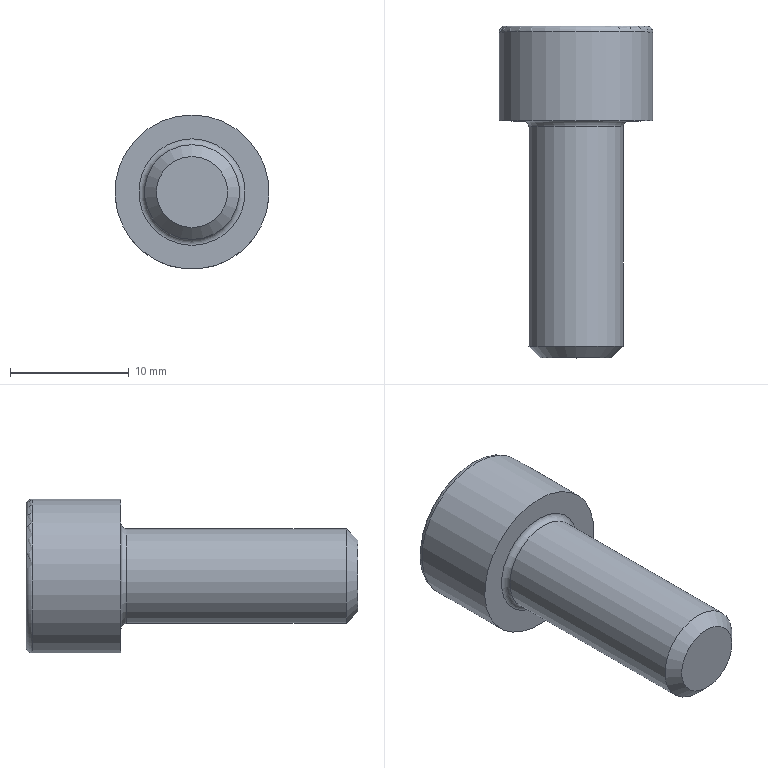Part | STEP file | SA10820 | 1 solid | 21 faces | box 13 x 28 x 13 mm | volume 1908 mm3 | plane 16 | cylinder 2 | torus 2 | cone 1 | commonest cylinder face diameters 8 x1 13 x1
STEP:
#1=CARTESIAN_POINT('',(0.,0.,4.5));
#2=VERTEX_POINT('',#1);
#3=CARTESIAN_POINT('',(0.,0.,0.));
#4=DIRECTION('',(0.,1.,0.));
#5=DIRECTION('',(0.,0.,1.));
#6=AXIS2_PLACEMENT_3D('',#3,#4,#5);
#7=CIRCLE('',#6,4.5);
#8=EDGE_CURVE('',#2,#2,#7,.T.);
#9=ORIENTED_EDGE('',*,*,#8,.T.);
#10=EDGE_LOOP('',(#9));
#11=FACE_BOUND('',#10,.T.);
#12=CARTESIAN_POINT('',(0.,0.,6.5));
#13=VERTEX_POINT('',#12);
#14=CARTESIAN_POINT('',(0.,0.,0.));
#15=DIRECTION('',(0.,1.,0.));
#16=DIRECTION('',(0.,0.,1.));
#17=AXIS2_PLACEMENT_3D('',#14,#15,#16);
#18=CIRCLE('',#17,6.5);
#19=EDGE_CURVE('',#13,#13,#18,.T.);
#20=ORIENTED_EDGE('',*,*,#19,.F.);
#21=EDGE_LOOP('',(#20));
#22=FACE_OUTER_BOUND('',#21,.T.);
#23=CARTESIAN_POINT('',(0.,0.,0.));
#24=DIRECTION('',(0.,1.,0.));
#25=DIRECTION('',(0.,0.,1.));
#26=AXIS2_PLACEMENT_3D('',#23,#24,#25);
#27=PLANE('',#26);
#28=ADVANCED_FACE('',(#11,#22),#27,.F.);
#29=CARTESIAN_POINT('',(0.,7.5,6.5));
#30=VERTEX_POINT('',#29);
#31=CARTESIAN_POINT('',(0.,7.5,0.));
#32=DIRECTION('',(0.,-1.,0.));
#33=DIRECTION('',(0.,0.,1.));
#34=AXIS2_PLACEMENT_3D('',#31,#32,#33);
#35=CIRCLE('',#34,6.5);
#36=EDGE_CURVE('',#30,#30,#35,.T.);
#37=ORIENTED_EDGE('',*,*,#36,.T.);
#38=EDGE_LOOP('',(#37));
#39=FACE_OUTER_BOUND('',#38,.T.);
#40=ORIENTED_EDGE('',*,*,#19,.T.);
#41=EDGE_LOOP('',(#40));
#42=FACE_OUTER_BOUND('',#41,.T.);
#43=CARTESIAN_POINT('',(0.,8.,0.));
#44=DIRECTION('',(0.,-1.,0.));
#45=DIRECTION('',(0.,0.,-1.));
#46=AXIS2_PLACEMENT_3D('',#43,#44,#45);
#47=CYLINDRICAL_SURFACE('',#46,6.5);
#48=ADVANCED_FACE('',(#39,#42),#47,.T.);
#49=CARTESIAN_POINT('',(0.,8.,6.));
#50=VERTEX_POINT('',#49);
#51=CARTESIAN_POINT('',(0.,8.,0.));
#52=DIRECTION('',(0.,1.,0.));
#53=DIRECTION('',(0.,0.,1.));
#54=AXIS2_PLACEMENT_3D('',#51,#52,#53);
#55=CIRCLE('',#54,6.);
#56=EDGE_CURVE('',#50,#50,#55,.T.);
#57=ORIENTED_EDGE('',*,*,#56,.T.);
#58=EDGE_LOOP('',(#57));
#59=FACE_OUTER_BOUND('',#58,.T.);
#60=CARTESIAN_POINT('',(3.464,8.,0.));
#61=VERTEX_POINT('',#60);
#62=CARTESIAN_POINT('',(1.732,8.,-3.));
#63=VERTEX_POINT('',#62);
#64=CARTESIAN_POINT('',(3.464,8.,0.));
#65=DIRECTION('',(-0.5,0.,-0.866));
#66=VECTOR('',#65,1000.);
#67=LINE('',#64,#66);
#68=EDGE_CURVE('',#61,#63,#67,.T.);
#69=ORIENTED_EDGE('',*,*,#68,.F.);
#70=CARTESIAN_POINT('',(1.732,8.,3.));
#71=VERTEX_POINT('',#70);
#72=CARTESIAN_POINT('',(1.732,8.,3.));
#73=DIRECTION('',(0.5,0.,-0.866));
#74=VECTOR('',#73,1000.);
#75=LINE('',#72,#74);
#76=EDGE_CURVE('',#71,#61,#75,.T.);
#77=ORIENTED_EDGE('',*,*,#76,.F.);
#78=CARTESIAN_POINT('',(-1.732,8.,3.));
#79=VERTEX_POINT('',#78);
#80=CARTESIAN_POINT('',(-1.732,8.,3.));
#81=DIRECTION('',(1.,0.,0.));
#82=VECTOR('',#81,1000.);
#83=LINE('',#80,#82);
#84=EDGE_CURVE('',#79,#71,#83,.T.);
#85=ORIENTED_EDGE('',*,*,#84,.F.);
#86=CARTESIAN_POINT('',(-3.464,8.,0.));
#87=VERTEX_POINT('',#86);
#88=CARTESIAN_POINT('',(-3.464,8.,0.));
#89=DIRECTION('',(0.5,0.,0.866));
#90=VECTOR('',#89,1000.);
#91=LINE('',#88,#90);
#92=EDGE_CURVE('',#87,#79,#91,.T.);
#93=ORIENTED_EDGE('',*,*,#92,.F.);
#94=CARTESIAN_POINT('',(-1.732,8.,-3.));
#95=VERTEX_POINT('',#94);
#96=CARTESIAN_POINT('',(-1.732,8.,-3.));
#97=DIRECTION('',(-0.5,0.,0.866));
#98=VECTOR('',#97,1000.);
#99=LINE('',#96,#98);
#100=EDGE_CURVE('',#95,#87,#99,.T.);
#101=ORIENTED_EDGE('',*,*,#100,.F.);
#102=CARTESIAN_POINT('',(1.732,8.,-3.));
#103=DIRECTION('',(-1.,0.,0.));
#104=VECTOR('',#103,1000.);
#105=LINE('',#102,#104);
#106=EDGE_CURVE('',#63,#95,#105,.T.);
#107=ORIENTED_EDGE('',*,*,#106,.F.);
#108=EDGE_LOOP('',(#69,#77,#85,#93,#101,#107));
#109=FACE_BOUND('',#108,.T.);
#110=CARTESIAN_POINT('',(0.,8.,0.));
#111=DIRECTION('',(0.,1.,0.));
#112=DIRECTION('',(0.,0.,1.));
#113=AXIS2_PLACEMENT_3D('',#110,#111,#112);
#114=PLANE('',#113);
#115=ADVANCED_FACE('',(#59,#109),#114,.T.);
#116=CARTESIAN_POINT('',(0.,-19.,-4.));
#117=VERTEX_POINT('',#116);
#118=CARTESIAN_POINT('',(0.,-19.,0.));
#119=DIRECTION('',(0.,1.,0.));
#120=DIRECTION('',(0.,0.,-1.));
#121=AXIS2_PLACEMENT_3D('',#118,#119,#120);
#122=CIRCLE('',#121,4.);
#123=EDGE_CURVE('',#117,#117,#122,.T.);
#124=ORIENTED_EDGE('',*,*,#123,.T.);
#125=EDGE_LOOP('',(#124));
#126=FACE_OUTER_BOUND('',#125,.T.);
#127=CARTESIAN_POINT('',(0.,-0.5,4.));
#128=VERTEX_POINT('',#127);
#129=CARTESIAN_POINT('',(0.,-0.5,0.));
#130=DIRECTION('',(0.,-1.,0.));
#131=DIRECTION('',(0.,0.,1.));
#132=AXIS2_PLACEMENT_3D('',#129,#130,#131);
#133=CIRCLE('',#132,4.);
#134=EDGE_CURVE('',#128,#128,#133,.T.);
#135=ORIENTED_EDGE('',*,*,#134,.T.);
#136=EDGE_LOOP('',(#135));
#137=FACE_OUTER_BOUND('',#136,.T.);
#138=CARTESIAN_POINT('',(0.,-20.,0.));
#139=DIRECTION('',(0.,1.,0.));
#140=DIRECTION('',(0.,0.,1.));
#141=AXIS2_PLACEMENT_3D('',#138,#139,#140);
#142=CYLINDRICAL_SURFACE('',#141,4.);
#143=ADVANCED_FACE('',(#126,#137),#142,.T.);
#144=CARTESIAN_POINT('',(0.,-20.,-3.));
#145=VERTEX_POINT('',#144);
#146=CARTESIAN_POINT('',(0.,-20.,0.));
#147=DIRECTION('',(0.,-1.,0.));
#148=DIRECTION('',(0.,0.,-1.));
#149=AXIS2_PLACEMENT_3D('',#146,#147,#148);
#150=CIRCLE('',#149,3.);
#151=EDGE_CURVE('',#145,#145,#150,.T.);
#152=ORIENTED_EDGE('',*,*,#151,.T.);
#153=EDGE_LOOP('',(#152));
#154=FACE_OUTER_BOUND('',#153,.T.);
#155=CARTESIAN_POINT('',(0.,-20.,0.));
#156=DIRECTION('',(0.,-1.,0.));
#157=DIRECTION('',(0.,0.,-1.));
#158=AXIS2_PLACEMENT_3D('',#155,#156,#157);
#159=PLANE('',#158);
#160=ADVANCED_FACE('',(#154),#159,.T.);
#161=CARTESIAN_POINT('',(1.732,4.,-3.));
#162=VERTEX_POINT('',#161);
#163=CARTESIAN_POINT('',(1.732,3.,-3.));
#164=DIRECTION('',(0.,1.,0.));
#165=VECTOR('',#164,1000.);
#166=LINE('',#163,#165);
#167=EDGE_CURVE('',#162,#63,#166,.T.);
#168=ORIENTED_EDGE('',*,*,#167,.F.);
#169=CARTESIAN_POINT('',(3.464,4.,0.));
#170=VERTEX_POINT('',#169);
#171=CARTESIAN_POINT('',(3.464,4.,0.));
#172=DIRECTION('',(0.5,0.,0.866));
#173=VECTOR('',#172,1000.);
#174=LINE('',#171,#173);
#175=EDGE_CURVE('',#162,#170,#174,.T.);
#176=ORIENTED_EDGE('',*,*,#175,.T.);
#177=CARTESIAN_POINT('',(3.464,3.,0.));
#178=DIRECTION('',(0.,1.,0.));
#179=VECTOR('',#178,1000.);
#180=LINE('',#177,#179);
#181=EDGE_CURVE('',#170,#61,#180,.T.);
#182=ORIENTED_EDGE('',*,*,#181,.T.);
#183=ORIENTED_EDGE('',*,*,#68,.T.);
#184=EDGE_LOOP('',(#168,#176,#182,#183));
#185=FACE_OUTER_BOUND('',#184,.T.);
#186=CARTESIAN_POINT('',(3.464,3.,0.));
#187=DIRECTION('',(0.866,0.,-0.5));
#188=DIRECTION('',(-0.5,0.,-0.866));
#189=AXIS2_PLACEMENT_3D('',#186,#187,#188);
#190=PLANE('',#189);
#191=ADVANCED_FACE('',(#185),#190,.F.);
#192=ORIENTED_EDGE('',*,*,#181,.F.);
#193=CARTESIAN_POINT('',(1.732,4.,3.));
#194=VERTEX_POINT('',#193);
#195=CARTESIAN_POINT('',(1.732,4.,3.));
#196=DIRECTION('',(-0.5,0.,0.866));
#197=VECTOR('',#196,1000.);
#198=LINE('',#195,#197);
#199=EDGE_CURVE('',#170,#194,#198,.T.);
#200=ORIENTED_EDGE('',*,*,#199,.T.);
#201=CARTESIAN_POINT('',(1.732,3.,3.));
#202=DIRECTION('',(0.,1.,0.));
#203=VECTOR('',#202,1000.);
#204=LINE('',#201,#203);
#205=EDGE_CURVE('',#194,#71,#204,.T.);
#206=ORIENTED_EDGE('',*,*,#205,.T.);
#207=ORIENTED_EDGE('',*,*,#76,.T.);
#208=EDGE_LOOP('',(#192,#200,#206,#207));
#209=FACE_OUTER_BOUND('',#208,.T.);
#210=CARTESIAN_POINT('',(1.732,3.,3.));
#211=DIRECTION('',(0.866,0.,0.5));
#212=DIRECTION('',(0.5,0.,-0.866));
#213=AXIS2_PLACEMENT_3D('',#210,#211,#212);
#214=PLANE('',#213);
#215=ADVANCED_FACE('',(#209),#214,.F.);
#216=ORIENTED_EDGE('',*,*,#205,.F.);
#217=CARTESIAN_POINT('',(-1.732,4.,3.));
#218=VERTEX_POINT('',#217);
#219=CARTESIAN_POINT('',(-1.732,4.,3.));
#220=DIRECTION('',(-1.,0.,0.));
#221=VECTOR('',#220,1000.);
#222=LINE('',#219,#221);
#223=EDGE_CURVE('',#194,#218,#222,.T.);
#224=ORIENTED_EDGE('',*,*,#223,.T.);
#225=CARTESIAN_POINT('',(-1.732,3.,3.));
#226=DIRECTION('',(0.,1.,0.));
#227=VECTOR('',#226,1000.);
#228=LINE('',#225,#227);
#229=EDGE_CURVE('',#218,#79,#228,.T.);
#230=ORIENTED_EDGE('',*,*,#229,.T.);
#231=ORIENTED_EDGE('',*,*,#84,.T.);
#232=EDGE_LOOP('',(#216,#224,#230,#231));
#233=FACE_OUTER_BOUND('',#232,.T.);
#234=CARTESIAN_POINT('',(-1.732,3.,3.));
#235=DIRECTION('',(0.,0.,1.));
#236=DIRECTION('',(1.,0.,0.));
#237=AXIS2_PLACEMENT_3D('',#234,#235,#236);
#238=PLANE('',#237);
#239=ADVANCED_FACE('',(#233),#238,.F.);
#240=ORIENTED_EDGE('',*,*,#229,.F.);
#241=CARTESIAN_POINT('',(-3.464,4.,0.));
#242=VERTEX_POINT('',#241);
#243=CARTESIAN_POINT('',(-3.464,4.,0.));
#244=DIRECTION('',(-0.5,0.,-0.866));
#245=VECTOR('',#244,1000.);
#246=LINE('',#243,#245);
#247=EDGE_CURVE('',#218,#242,#246,.T.);
#248=ORIENTED_EDGE('',*,*,#247,.T.);
#249=CARTESIAN_POINT('',(-3.464,3.,0.));
#250=DIRECTION('',(0.,1.,0.));
#251=VECTOR('',#250,1000.);
#252=LINE('',#249,#251);
#253=EDGE_CURVE('',#242,#87,#252,.T.);
#254=ORIENTED_EDGE('',*,*,#253,.T.);
#255=ORIENTED_EDGE('',*,*,#92,.T.);
#256=EDGE_LOOP('',(#240,#248,#254,#255));
#257=FACE_OUTER_BOUND('',#256,.T.);
#258=CARTESIAN_POINT('',(-3.464,3.,0.));
#259=DIRECTION('',(-0.866,0.,0.5));
#260=DIRECTION('',(0.5,0.,0.866));
#261=AXIS2_PLACEMENT_3D('',#258,#259,#260);
#262=PLANE('',#261);
#263=ADVANCED_FACE('',(#257),#262,.F.);
#264=ORIENTED_EDGE('',*,*,#253,.F.);
#265=CARTESIAN_POINT('',(-1.732,4.,-3.));
#266=VERTEX_POINT('',#265);
#267=CARTESIAN_POINT('',(-1.732,4.,-3.));
#268=DIRECTION('',(0.5,0.,-0.866));
#269=VECTOR('',#268,1000.);
#270=LINE('',#267,#269);
#271=EDGE_CURVE('',#242,#266,#270,.T.);
#272=ORIENTED_EDGE('',*,*,#271,.T.);
#273=CARTESIAN_POINT('',(-1.732,3.,-3.));
#274=DIRECTION('',(0.,1.,0.));
#275=VECTOR('',#274,1000.);
#276=LINE('',#273,#275);
#277=EDGE_CURVE('',#266,#95,#276,.T.);
#278=ORIENTED_EDGE('',*,*,#277,.T.);
#279=ORIENTED_EDGE('',*,*,#100,.T.);
#280=EDGE_LOOP('',(#264,#272,#278,#279));
#281=FACE_OUTER_BOUND('',#280,.T.);
#282=CARTESIAN_POINT('',(-1.732,3.,-3.));
#283=DIRECTION('',(-0.866,0.,-0.5));
#284=DIRECTION('',(-0.5,0.,0.866));
#285=AXIS2_PLACEMENT_3D('',#282,#283,#284);
#286=PLANE('',#285);
#287=ADVANCED_FACE('',(#281),#286,.F.);
#288=ORIENTED_EDGE('',*,*,#277,.F.);
#289=CARTESIAN_POINT('',(1.732,4.,-3.));
#290=DIRECTION('',(1.,0.,0.));
#291=VECTOR('',#290,1000.);
#292=LINE('',#289,#291);
#293=EDGE_CURVE('',#266,#162,#292,.T.);
#294=ORIENTED_EDGE('',*,*,#293,.T.);
#295=ORIENTED_EDGE('',*,*,#167,.T.);
#296=ORIENTED_EDGE('',*,*,#106,.T.);
#297=EDGE_LOOP('',(#288,#294,#295,#296));
#298=FACE_OUTER_BOUND('',#297,.T.);
#299=CARTESIAN_POINT('',(1.732,3.,-3.));
#300=DIRECTION('',(0.,0.,-1.));
#301=DIRECTION('',(-1.,0.,0.));
#302=AXIS2_PLACEMENT_3D('',#299,#300,#301);
#303=PLANE('',#302);
#304=ADVANCED_FACE('',(#298),#303,.F.);
#305=CARTESIAN_POINT('',(-1.155,3.,2.));
#306=VERTEX_POINT('',#305);
#307=CARTESIAN_POINT('',(1.155,3.,2.));
#308=VERTEX_POINT('',#307);
#309=CARTESIAN_POINT('',(0.,3.,2.));
#310=DIRECTION('',(1.,0.,0.));
#311=VECTOR('',#310,1000.);
#312=LINE('',#309,#311);
#313=EDGE_CURVE('',#306,#308,#312,.T.);
#314=ORIENTED_EDGE('',*,*,#313,.T.);
#315=CARTESIAN_POINT('',(2.309,3.,0.));
#316=VERTEX_POINT('',#315);
#317=CARTESIAN_POINT('',(4.33,3.,-3.5));
#318=DIRECTION('',(0.5,0.,-0.866));
#319=VECTOR('',#318,1000.);
#320=LINE('',#317,#319);
#321=EDGE_CURVE('',#308,#316,#320,.T.);
#322=ORIENTED_EDGE('',*,*,#321,.T.);
#323=CARTESIAN_POINT('',(1.155,3.,-2.));
#324=VERTEX_POINT('',#323);
#325=CARTESIAN_POINT('',(-0.866,3.,-5.5));
#326=DIRECTION('',(-0.5,0.,-0.866));
#327=VECTOR('',#326,1000.);
#328=LINE('',#325,#327);
#329=EDGE_CURVE('',#316,#324,#328,.T.);
#330=ORIENTED_EDGE('',*,*,#329,.T.);
#331=CARTESIAN_POINT('',(-1.155,3.,-2.));
#332=VERTEX_POINT('',#331);
#333=CARTESIAN_POINT('',(0.,3.,-2.));
#334=DIRECTION('',(-1.,0.,0.));
#335=VECTOR('',#334,1000.);
#336=LINE('',#333,#335);
#337=EDGE_CURVE('',#324,#332,#336,.T.);
#338=ORIENTED_EDGE('',*,*,#337,.T.);
#339=CARTESIAN_POINT('',(-2.309,3.,0.));
#340=VERTEX_POINT('',#339);
#341=CARTESIAN_POINT('',(0.866,3.,-5.5));
#342=DIRECTION('',(-0.5,0.,0.866));
#343=VECTOR('',#342,1000.);
#344=LINE('',#341,#343);
#345=EDGE_CURVE('',#332,#340,#344,.T.);
#346=ORIENTED_EDGE('',*,*,#345,.T.);
#347=CARTESIAN_POINT('',(-4.33,3.,-3.5));
#348=DIRECTION('',(0.5,0.,0.866));
#349=VECTOR('',#348,1000.);
#350=LINE('',#347,#349);
#351=EDGE_CURVE('',#340,#306,#350,.T.);
#352=ORIENTED_EDGE('',*,*,#351,.T.);
#353=EDGE_LOOP('',(#314,#322,#330,#338,#346,#352));
#354=FACE_OUTER_BOUND('',#353,.T.);
#355=CARTESIAN_POINT('',(0.,3.,-6.));
#356=DIRECTION('',(0.,1.,0.));
#357=DIRECTION('',(0.,0.,1.));
#358=AXIS2_PLACEMENT_3D('',#355,#356,#357);
#359=PLANE('',#358);
#360=ADVANCED_FACE('',(#354),#359,.T.);
#361=ORIENTED_EDGE('',*,*,#8,.F.);
#362=EDGE_LOOP('',(#361));
#363=FACE_OUTER_BOUND('',#362,.T.);
#364=ORIENTED_EDGE('',*,*,#134,.F.);
#365=EDGE_LOOP('',(#364));
#366=FACE_OUTER_BOUND('',#365,.T.);
#367=CARTESIAN_POINT('',(0.,-0.5,0.));
#368=DIRECTION('',(0.,1.,0.));
#369=DIRECTION('',(0.,0.,1.));
#370=AXIS2_PLACEMENT_3D('',#367,#368,#369);
#371=TOROIDAL_SURFACE('',#370,4.5,0.5);
#372=ADVANCED_FACE('',(#363,#366),#371,.F.);
#373=ORIENTED_EDGE('',*,*,#123,.F.);
#374=EDGE_LOOP('',(#373));
#375=FACE_OUTER_BOUND('',#374,.T.);
#376=ORIENTED_EDGE('',*,*,#151,.F.);
#377=EDGE_LOOP('',(#376));
#378=FACE_BOUND('',#377,.T.);
#379=CARTESIAN_POINT('',(0.,-20.,0.));
#380=DIRECTION('',(0.,1.,0.));
#381=DIRECTION('',(0.,0.,1.));
#382=AXIS2_PLACEMENT_3D('',#379,#380,#381);
#383=CONICAL_SURFACE('',#382,3.,0.7854);
#384=ADVANCED_FACE('',(#375,#378),#383,.T.);
#385=ORIENTED_EDGE('',*,*,#36,.F.);
#386=EDGE_LOOP('',(#385));
#387=FACE_OUTER_BOUND('',#386,.T.);
#388=ORIENTED_EDGE('',*,*,#56,.F.);
#389=EDGE_LOOP('',(#388));
#390=FACE_OUTER_BOUND('',#389,.T.);
#391=CARTESIAN_POINT('',(0.,7.5,0.));
#392=DIRECTION('',(0.,1.,0.));
#393=DIRECTION('',(0.,0.,1.));
#394=AXIS2_PLACEMENT_3D('',#391,#392,#393);
#395=TOROIDAL_SURFACE('',#394,6.,0.5);
#396=ADVANCED_FACE('',(#387,#390),#395,.T.);
#397=CARTESIAN_POINT('',(-1.732,4.,-3.));
#398=DIRECTION('',(0.378,-0.6547,0.6547));
#399=VECTOR('',#398,1000.);
#400=LINE('',#397,#399);
#401=EDGE_CURVE('',#266,#332,#400,.T.);
#402=ORIENTED_EDGE('',*,*,#401,.F.);
#403=ORIENTED_EDGE('',*,*,#271,.F.);
#404=CARTESIAN_POINT('',(-3.464,4.,0.));
#405=DIRECTION('',(-0.7559,0.6547,0.));
#406=VECTOR('',#405,1000.);
#407=LINE('',#404,#406);
#408=EDGE_CURVE('',#340,#242,#407,.T.);
#409=ORIENTED_EDGE('',*,*,#408,.F.);
#410=ORIENTED_EDGE('',*,*,#345,.F.);
#411=EDGE_LOOP('',(#402,#403,#409,#410));
#412=FACE_OUTER_BOUND('',#411,.T.);
#413=CARTESIAN_POINT('',(0.866,3.,-5.5));
#414=DIRECTION('',(-0.6124,-0.7071,-0.3536));
#415=DIRECTION('',(0.7559,-0.6547,0.));
#416=AXIS2_PLACEMENT_3D('',#413,#414,#415);
#417=PLANE('',#416);
#418=ADVANCED_FACE('',(#412),#417,.F.);
#419=ORIENTED_EDGE('',*,*,#408,.T.);
#420=ORIENTED_EDGE('',*,*,#247,.F.);
#421=CARTESIAN_POINT('',(-0.9897,2.714,1.714));
#422=DIRECTION('',(-0.378,0.6547,0.6547));
#423=VECTOR('',#422,1000.);
#424=LINE('',#421,#423);
#425=EDGE_CURVE('',#306,#218,#424,.T.);
#426=ORIENTED_EDGE('',*,*,#425,.F.);
#427=ORIENTED_EDGE('',*,*,#351,.F.);
#428=EDGE_LOOP('',(#419,#420,#426,#427));
#429=FACE_OUTER_BOUND('',#428,.T.);
#430=CARTESIAN_POINT('',(-4.33,3.,-3.5));
#431=DIRECTION('',(-0.6124,-0.7071,0.3536));
#432=DIRECTION('',(0.7559,-0.6547,0.));
#433=AXIS2_PLACEMENT_3D('',#430,#431,#432);
#434=PLANE('',#433);
#435=ADVANCED_FACE('',(#429),#434,.F.);
#436=ORIENTED_EDGE('',*,*,#401,.T.);
#437=ORIENTED_EDGE('',*,*,#337,.F.);
#438=CARTESIAN_POINT('',(0.9897,2.714,-1.714));
#439=DIRECTION('',(-0.378,-0.6547,0.6547));
#440=VECTOR('',#439,1000.);
#441=LINE('',#438,#440);
#442=EDGE_CURVE('',#162,#324,#441,.T.);
#443=ORIENTED_EDGE('',*,*,#442,.F.);
#444=ORIENTED_EDGE('',*,*,#293,.F.);
#445=EDGE_LOOP('',(#436,#437,#443,#444));
#446=FACE_OUTER_BOUND('',#445,.T.);
#447=CARTESIAN_POINT('',(0.,3.,-2.));
#448=DIRECTION('',(0.,-0.7071,-0.7071));
#449=DIRECTION('',(0.,0.7071,-0.7071));
#450=AXIS2_PLACEMENT_3D('',#447,#448,#449);
#451=PLANE('',#450);
#452=ADVANCED_FACE('',(#446),#451,.F.);
#453=ORIENTED_EDGE('',*,*,#425,.T.);
#454=ORIENTED_EDGE('',*,*,#223,.F.);
#455=CARTESIAN_POINT('',(0.2474,1.429,0.4286));
#456=DIRECTION('',(0.378,0.6547,0.6547));
#457=VECTOR('',#456,1000.);
#458=LINE('',#455,#457);
#459=EDGE_CURVE('',#308,#194,#458,.T.);
#460=ORIENTED_EDGE('',*,*,#459,.F.);
#461=ORIENTED_EDGE('',*,*,#313,.F.);
#462=EDGE_LOOP('',(#453,#454,#460,#461));
#463=FACE_OUTER_BOUND('',#462,.T.);
#464=CARTESIAN_POINT('',(0.,3.,2.));
#465=DIRECTION('',(0.,-0.7071,0.7071));
#466=DIRECTION('',(0.,-0.7071,-0.7071));
#467=AXIS2_PLACEMENT_3D('',#464,#465,#466);
#468=PLANE('',#467);
#469=ADVANCED_FACE('',(#463),#468,.F.);
#470=ORIENTED_EDGE('',*,*,#442,.T.);
#471=ORIENTED_EDGE('',*,*,#329,.F.);
#472=CARTESIAN_POINT('',(3.464,4.,0.));
#473=DIRECTION('',(-0.7559,-0.6547,0.));
#474=VECTOR('',#473,1000.);
#475=LINE('',#472,#474);
#476=EDGE_CURVE('',#170,#316,#475,.T.);
#477=ORIENTED_EDGE('',*,*,#476,.F.);
#478=ORIENTED_EDGE('',*,*,#175,.F.);
#479=EDGE_LOOP('',(#470,#471,#477,#478));
#480=FACE_OUTER_BOUND('',#479,.T.);
#481=CARTESIAN_POINT('',(-0.866,3.,-5.5));
#482=DIRECTION('',(0.6124,-0.7071,-0.3536));
#483=DIRECTION('',(0.7559,0.6547,0.));
#484=AXIS2_PLACEMENT_3D('',#481,#482,#483);
#485=PLANE('',#484);
#486=ADVANCED_FACE('',(#480),#485,.F.);
#487=ORIENTED_EDGE('',*,*,#459,.T.);
#488=ORIENTED_EDGE('',*,*,#199,.F.);
#489=ORIENTED_EDGE('',*,*,#476,.T.);
#490=ORIENTED_EDGE('',*,*,#321,.F.);
#491=EDGE_LOOP('',(#487,#488,#489,#490));
#492=FACE_OUTER_BOUND('',#491,.T.);
#493=CARTESIAN_POINT('',(4.33,3.,-3.5));
#494=DIRECTION('',(0.6124,-0.7071,0.3536));
#495=DIRECTION('',(0.7559,0.6547,0.));
#496=AXIS2_PLACEMENT_3D('',#493,#494,#495);
#497=PLANE('',#496);
#498=ADVANCED_FACE('',(#492),#497,.F.);
#499=CLOSED_SHELL('',(#28,#48,#115,#143,#160,#191,#215,#239,#263,#287,#304,#360,#372,#384,#396,#418,#435,#452,#469,#486,#498));
#500=MANIFOLD_SOLID_BREP('',#499);
#501=CARTESIAN_POINT('',(0.,0.,0.));
#502=DIRECTION('',(0.,0.,1.));
#503=DIRECTION('',(1.,0.,0.));
#504=AXIS2_PLACEMENT_3D('',#501,#502,#503);
#505=(LENGTH_UNIT()NAMED_UNIT(*)SI_UNIT(.MILLI.,.METRE.));
#506=UNCERTAINTY_MEASURE_WITH_UNIT(LENGTH_MEASURE(0.00001),#505,'','');
#507=(NAMED_UNIT(*)PLANE_ANGLE_UNIT()SI_UNIT($,.RADIAN.));
#508=(NAMED_UNIT(*)SI_UNIT($,.STERADIAN.)SOLID_ANGLE_UNIT());
#509=(GEOMETRIC_REPRESENTATION_CONTEXT(3)GLOBAL_UNCERTAINTY_ASSIGNED_CONTEXT((#506))GLOBAL_UNIT_ASSIGNED_CONTEXT((#505,#507,#508))REPRESENTATION_CONTEXT('',''));
#510=ADVANCED_BREP_SHAPE_REPRESENTATION('',(#500,#504),#509);